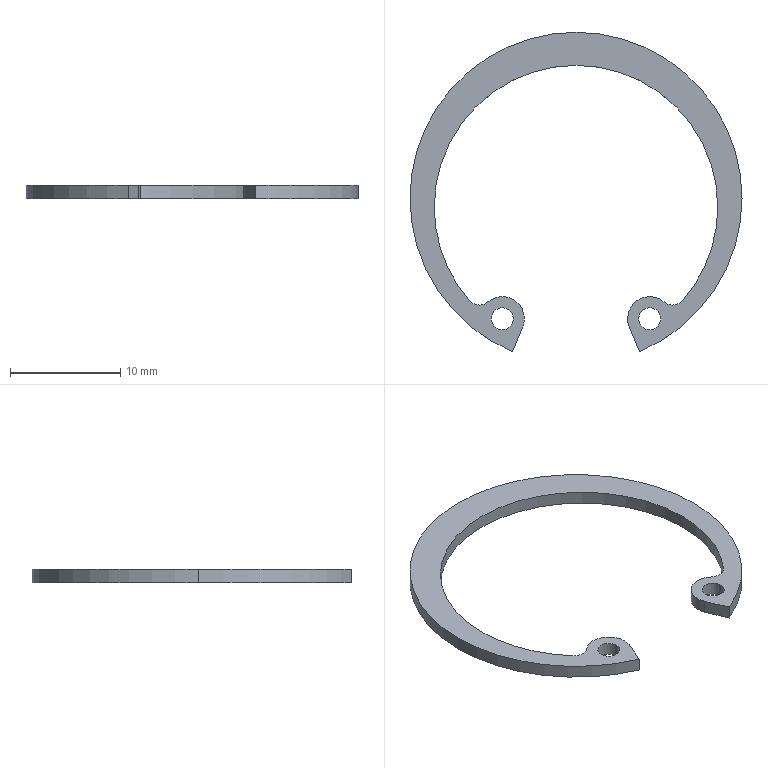Part | SolidWorks | features BaseBody 1 | 1 solid | 19 faces | box 30.1 x 28.954 x 1.2 mm | volume 227.232 mm3 | cylinder 15 | plane 4 | commonest cylinder face diameters 2 x4 4 x3 25.7 x3 30.1 x3 2.4 x2
STEP:
#1=CARTESIAN_POINT('',(15.05,0.,-1.2));
#2=VERTEX_POINT('',#1);
#3=CARTESIAN_POINT('',(-15.05,0.,-1.2));
#4=VERTEX_POINT('',#3);
#5=CARTESIAN_POINT('',(0.,0.,-1.2));
#6=DIRECTION('',(0.,0.,1.));
#7=DIRECTION('',(1.,0.,0.));
#8=AXIS2_PLACEMENT_3D('',#5,#6,#7);
#9=CIRCLE('',#8,15.05);
#10=EDGE_CURVE('',#2,#4,#9,.T.);
#11=ORIENTED_EDGE('',*,*,#10,.T.);
#12=CARTESIAN_POINT('',(-15.05,0.,0.));
#13=VERTEX_POINT('',#12);
#14=CARTESIAN_POINT('',(-15.05,0.,-1.2));
#15=DIRECTION('',(0.,0.,1.));
#16=VECTOR('',#15,1000.);
#17=LINE('',#14,#16);
#18=EDGE_CURVE('',#4,#13,#17,.T.);
#19=ORIENTED_EDGE('',*,*,#18,.T.);
#20=CARTESIAN_POINT('',(15.05,0.,0.));
#21=VERTEX_POINT('',#20);
#22=CARTESIAN_POINT('',(0.,0.,0.));
#23=DIRECTION('',(0.,0.,-1.));
#24=DIRECTION('',(1.,0.,0.));
#25=AXIS2_PLACEMENT_3D('',#22,#23,#24);
#26=CIRCLE('',#25,15.05);
#27=EDGE_CURVE('',#13,#21,#26,.T.);
#28=ORIENTED_EDGE('',*,*,#27,.T.);
#29=CARTESIAN_POINT('',(15.05,0.,-1.2));
#30=DIRECTION('',(0.,0.,1.));
#31=VECTOR('',#30,1000.);
#32=LINE('',#29,#31);
#33=EDGE_CURVE('',#2,#21,#32,.T.);
#34=ORIENTED_EDGE('',*,*,#33,.F.);
#35=EDGE_LOOP('',(#11,#19,#28,#34));
#36=FACE_OUTER_BOUND('',#35,.T.);
#37=CARTESIAN_POINT('',(0.,0.,-1.2));
#38=DIRECTION('',(0.,0.,1.));
#39=DIRECTION('',(1.,0.,0.));
#40=AXIS2_PLACEMENT_3D('',#37,#38,#39);
#41=CYLINDRICAL_SURFACE('',#40,15.05);
#42=ADVANCED_FACE('',(#36),#41,.T.);
#43=CARTESIAN_POINT('',(5.759,-13.904,-1.2));
#44=VERTEX_POINT('',#43);
#45=CARTESIAN_POINT('',(0.,0.,-1.2));
#46=DIRECTION('',(0.,0.,1.));
#47=DIRECTION('',(1.,0.,0.));
#48=AXIS2_PLACEMENT_3D('',#45,#46,#47);
#49=CIRCLE('',#48,15.05);
#50=EDGE_CURVE('',#44,#2,#49,.T.);
#51=ORIENTED_EDGE('',*,*,#50,.T.);
#52=ORIENTED_EDGE('',*,*,#33,.T.);
#53=CARTESIAN_POINT('',(5.759,-13.904,0.));
#54=VERTEX_POINT('',#53);
#55=CARTESIAN_POINT('',(0.,0.,0.));
#56=DIRECTION('',(0.,0.,-1.));
#57=DIRECTION('',(1.,0.,0.));
#58=AXIS2_PLACEMENT_3D('',#55,#56,#57);
#59=CIRCLE('',#58,15.05);
#60=EDGE_CURVE('',#21,#54,#59,.T.);
#61=ORIENTED_EDGE('',*,*,#60,.T.);
#62=CARTESIAN_POINT('',(5.759,-13.904,-1.2));
#63=DIRECTION('',(0.,0.,-1.));
#64=VECTOR('',#63,1000.);
#65=LINE('',#62,#64);
#66=EDGE_CURVE('',#54,#44,#65,.T.);
#67=ORIENTED_EDGE('',*,*,#66,.T.);
#68=EDGE_LOOP('',(#51,#52,#61,#67));
#69=FACE_OUTER_BOUND('',#68,.T.);
#70=CARTESIAN_POINT('',(0.,0.,-1.2));
#71=DIRECTION('',(0.,0.,1.));
#72=DIRECTION('',(1.,0.,0.));
#73=AXIS2_PLACEMENT_3D('',#70,#71,#72);
#74=CYLINDRICAL_SURFACE('',#73,15.05);
#75=ADVANCED_FACE('',(#69),#74,.T.);
#76=CARTESIAN_POINT('',(-9.663,-9.27,-1.2));
#77=VERTEX_POINT('',#76);
#78=CARTESIAN_POINT('',(-12.85,-0.8,-1.2));
#79=VERTEX_POINT('',#78);
#80=CARTESIAN_POINT('',(0.,-0.8,-1.2));
#81=DIRECTION('',(0.,0.,-1.));
#82=DIRECTION('',(1.,0.,0.));
#83=AXIS2_PLACEMENT_3D('',#80,#81,#82);
#84=CIRCLE('',#83,12.85);
#85=EDGE_CURVE('',#77,#79,#84,.T.);
#86=ORIENTED_EDGE('',*,*,#85,.T.);
#87=CARTESIAN_POINT('',(-12.85,-0.8,0.));
#88=VERTEX_POINT('',#87);
#89=CARTESIAN_POINT('',(-12.85,-0.8,-1.2));
#90=DIRECTION('',(0.,0.,1.));
#91=VECTOR('',#90,1000.);
#92=LINE('',#89,#91);
#93=EDGE_CURVE('',#79,#88,#92,.T.);
#94=ORIENTED_EDGE('',*,*,#93,.T.);
#95=CARTESIAN_POINT('',(-9.663,-9.27,0.));
#96=VERTEX_POINT('',#95);
#97=CARTESIAN_POINT('',(0.,-0.8,0.));
#98=DIRECTION('',(0.,0.,-1.));
#99=DIRECTION('',(1.,0.,0.));
#100=AXIS2_PLACEMENT_3D('',#97,#98,#99);
#101=CIRCLE('',#100,12.85);
#102=EDGE_CURVE('',#96,#88,#101,.T.);
#103=ORIENTED_EDGE('',*,*,#102,.F.);
#104=CARTESIAN_POINT('',(-9.663,-9.27,-1.2));
#105=DIRECTION('',(0.,0.,1.));
#106=VECTOR('',#105,1000.);
#107=LINE('',#104,#106);
#108=EDGE_CURVE('',#77,#96,#107,.T.);
#109=ORIENTED_EDGE('',*,*,#108,.F.);
#110=EDGE_LOOP('',(#86,#94,#103,#109));
#111=FACE_OUTER_BOUND('',#110,.T.);
#112=CARTESIAN_POINT('',(0.,-0.8,-1.2));
#113=DIRECTION('',(0.,0.,1.));
#114=DIRECTION('',(1.,0.,0.));
#115=AXIS2_PLACEMENT_3D('',#112,#113,#114);
#116=CYLINDRICAL_SURFACE('',#115,12.85);
#117=ADVANCED_FACE('',(#111),#116,.F.);
#118=ORIENTED_EDGE('',*,*,#93,.F.);
#119=CARTESIAN_POINT('',(12.85,-0.8,-1.2));
#120=VERTEX_POINT('',#119);
#121=CARTESIAN_POINT('',(0.,-0.8,-1.2));
#122=DIRECTION('',(0.,0.,-1.));
#123=DIRECTION('',(1.,0.,0.));
#124=AXIS2_PLACEMENT_3D('',#121,#122,#123);
#125=CIRCLE('',#124,12.85);
#126=EDGE_CURVE('',#79,#120,#125,.T.);
#127=ORIENTED_EDGE('',*,*,#126,.T.);
#128=CARTESIAN_POINT('',(12.85,-0.8,0.));
#129=VERTEX_POINT('',#128);
#130=CARTESIAN_POINT('',(12.85,-0.8,-1.2));
#131=DIRECTION('',(0.,0.,1.));
#132=VECTOR('',#131,1000.);
#133=LINE('',#130,#132);
#134=EDGE_CURVE('',#120,#129,#133,.T.);
#135=ORIENTED_EDGE('',*,*,#134,.T.);
#136=CARTESIAN_POINT('',(0.,-0.8,0.));
#137=DIRECTION('',(0.,0.,-1.));
#138=DIRECTION('',(1.,0.,0.));
#139=AXIS2_PLACEMENT_3D('',#136,#137,#138);
#140=CIRCLE('',#139,12.85);
#141=EDGE_CURVE('',#88,#129,#140,.T.);
#142=ORIENTED_EDGE('',*,*,#141,.F.);
#143=EDGE_LOOP('',(#118,#127,#135,#142));
#144=FACE_OUTER_BOUND('',#143,.T.);
#145=CARTESIAN_POINT('',(0.,-0.8,-1.2));
#146=DIRECTION('',(0.,0.,1.));
#147=DIRECTION('',(1.,0.,0.));
#148=AXIS2_PLACEMENT_3D('',#145,#146,#147);
#149=CYLINDRICAL_SURFACE('',#148,12.85);
#150=ADVANCED_FACE('',(#144),#149,.F.);
#151=CARTESIAN_POINT('',(-4.838,-11.68,-1.2));
#152=VERTEX_POINT('',#151);
#153=CARTESIAN_POINT('',(-4.686,-10.915,-1.2));
#154=VERTEX_POINT('',#153);
#155=CARTESIAN_POINT('',(-6.686,-10.915,-1.2));
#156=DIRECTION('',(0.,0.,1.));
#157=DIRECTION('',(1.,0.,0.));
#158=AXIS2_PLACEMENT_3D('',#155,#156,#157);
#159=CIRCLE('',#158,2.);
#160=EDGE_CURVE('',#152,#154,#159,.T.);
#161=ORIENTED_EDGE('',*,*,#160,.T.);
#162=CARTESIAN_POINT('',(-4.686,-10.915,0.));
#163=VERTEX_POINT('',#162);
#164=CARTESIAN_POINT('',(-4.686,-10.915,-1.2));
#165=DIRECTION('',(0.,0.,1.));
#166=VECTOR('',#165,1000.);
#167=LINE('',#164,#166);
#168=EDGE_CURVE('',#154,#163,#167,.T.);
#169=ORIENTED_EDGE('',*,*,#168,.T.);
#170=CARTESIAN_POINT('',(-4.838,-11.68,0.));
#171=VERTEX_POINT('',#170);
#172=CARTESIAN_POINT('',(-6.686,-10.915,0.));
#173=DIRECTION('',(0.,0.,-1.));
#174=DIRECTION('',(1.,0.,0.));
#175=AXIS2_PLACEMENT_3D('',#172,#173,#174);
#176=CIRCLE('',#175,2.);
#177=EDGE_CURVE('',#163,#171,#176,.T.);
#178=ORIENTED_EDGE('',*,*,#177,.T.);
#179=CARTESIAN_POINT('',(-4.838,-11.68,-1.2));
#180=DIRECTION('',(0.,0.,-1.));
#181=VECTOR('',#180,1000.);
#182=LINE('',#179,#181);
#183=EDGE_CURVE('',#171,#152,#182,.T.);
#184=ORIENTED_EDGE('',*,*,#183,.T.);
#185=EDGE_LOOP('',(#161,#169,#178,#184));
#186=FACE_OUTER_BOUND('',#185,.T.);
#187=CARTESIAN_POINT('',(-6.686,-10.915,-1.2));
#188=DIRECTION('',(0.,0.,1.));
#189=DIRECTION('',(1.,0.,0.));
#190=AXIS2_PLACEMENT_3D('',#187,#188,#189);
#191=CYLINDRICAL_SURFACE('',#190,2.);
#192=ADVANCED_FACE('',(#186),#191,.T.);
#193=CARTESIAN_POINT('',(7.686,-10.915,-1.2));
#194=VERTEX_POINT('',#193);
#195=CARTESIAN_POINT('',(5.686,-10.915,-1.2));
#196=VERTEX_POINT('',#195);
#197=CARTESIAN_POINT('',(6.686,-10.915,-1.2));
#198=DIRECTION('',(0.,0.,-1.));
#199=DIRECTION('',(1.,0.,0.));
#200=AXIS2_PLACEMENT_3D('',#197,#198,#199);
#201=CIRCLE('',#200,1.);
#202=EDGE_CURVE('',#194,#196,#201,.T.);
#203=ORIENTED_EDGE('',*,*,#202,.T.);
#204=CARTESIAN_POINT('',(5.686,-10.915,0.));
#205=VERTEX_POINT('',#204);
#206=CARTESIAN_POINT('',(5.686,-10.915,-1.2));
#207=DIRECTION('',(0.,0.,1.));
#208=VECTOR('',#207,1000.);
#209=LINE('',#206,#208);
#210=EDGE_CURVE('',#196,#205,#209,.T.);
#211=ORIENTED_EDGE('',*,*,#210,.T.);
#212=CARTESIAN_POINT('',(7.686,-10.915,0.));
#213=VERTEX_POINT('',#212);
#214=CARTESIAN_POINT('',(6.686,-10.915,0.));
#215=DIRECTION('',(0.,0.,-1.));
#216=DIRECTION('',(1.,0.,0.));
#217=AXIS2_PLACEMENT_3D('',#214,#215,#216);
#218=CIRCLE('',#217,1.);
#219=EDGE_CURVE('',#213,#205,#218,.T.);
#220=ORIENTED_EDGE('',*,*,#219,.F.);
#221=CARTESIAN_POINT('',(7.686,-10.915,-1.2));
#222=DIRECTION('',(0.,0.,1.));
#223=VECTOR('',#222,1000.);
#224=LINE('',#221,#223);
#225=EDGE_CURVE('',#194,#213,#224,.T.);
#226=ORIENTED_EDGE('',*,*,#225,.F.);
#227=EDGE_LOOP('',(#203,#211,#220,#226));
#228=FACE_OUTER_BOUND('',#227,.T.);
#229=CARTESIAN_POINT('',(6.686,-10.915,-1.2));
#230=DIRECTION('',(0.,0.,1.));
#231=DIRECTION('',(1.,0.,0.));
#232=AXIS2_PLACEMENT_3D('',#229,#230,#231);
#233=CYLINDRICAL_SURFACE('',#232,1.);
#234=ADVANCED_FACE('',(#228),#233,.F.);
#235=CARTESIAN_POINT('',(-5.686,-10.915,-1.2));
#236=VERTEX_POINT('',#235);
#237=CARTESIAN_POINT('',(-7.686,-10.915,-1.2));
#238=VERTEX_POINT('',#237);
#239=CARTESIAN_POINT('',(-6.686,-10.915,-1.2));
#240=DIRECTION('',(0.,0.,-1.));
#241=DIRECTION('',(1.,0.,0.));
#242=AXIS2_PLACEMENT_3D('',#239,#240,#241);
#243=CIRCLE('',#242,1.);
#244=EDGE_CURVE('',#236,#238,#243,.T.);
#245=ORIENTED_EDGE('',*,*,#244,.T.);
#246=CARTESIAN_POINT('',(-7.686,-10.915,0.));
#247=VERTEX_POINT('',#246);
#248=CARTESIAN_POINT('',(-7.686,-10.915,-1.2));
#249=DIRECTION('',(0.,0.,1.));
#250=VECTOR('',#249,1000.);
#251=LINE('',#248,#250);
#252=EDGE_CURVE('',#238,#247,#251,.T.);
#253=ORIENTED_EDGE('',*,*,#252,.T.);
#254=CARTESIAN_POINT('',(-5.686,-10.915,0.));
#255=VERTEX_POINT('',#254);
#256=CARTESIAN_POINT('',(-6.686,-10.915,0.));
#257=DIRECTION('',(0.,0.,-1.));
#258=DIRECTION('',(1.,0.,0.));
#259=AXIS2_PLACEMENT_3D('',#256,#257,#258);
#260=CIRCLE('',#259,1.);
#261=EDGE_CURVE('',#255,#247,#260,.T.);
#262=ORIENTED_EDGE('',*,*,#261,.F.);
#263=CARTESIAN_POINT('',(-5.686,-10.915,-1.2));
#264=DIRECTION('',(0.,0.,1.));
#265=VECTOR('',#264,1000.);
#266=LINE('',#263,#265);
#267=EDGE_CURVE('',#236,#255,#266,.T.);
#268=ORIENTED_EDGE('',*,*,#267,.F.);
#269=EDGE_LOOP('',(#245,#253,#262,#268));
#270=FACE_OUTER_BOUND('',#269,.T.);
#271=CARTESIAN_POINT('',(-6.686,-10.915,-1.2));
#272=DIRECTION('',(0.,0.,1.));
#273=DIRECTION('',(1.,0.,0.));
#274=AXIS2_PLACEMENT_3D('',#271,#272,#273);
#275=CYLINDRICAL_SURFACE('',#274,1.);
#276=ADVANCED_FACE('',(#270),#275,.F.);
#277=CARTESIAN_POINT('',(4.838,-11.68,-1.2));
#278=VERTEX_POINT('',#277);
#279=CARTESIAN_POINT('',(4.838,-11.68,-1.2));
#280=DIRECTION('',(0.3827,-0.9239,0.));
#281=VECTOR('',#280,1000.);
#282=LINE('',#279,#281);
#283=EDGE_CURVE('',#278,#44,#282,.T.);
#284=ORIENTED_EDGE('',*,*,#283,.F.);
#285=CARTESIAN_POINT('',(7.983,-9.393,-1.2));
#286=VERTEX_POINT('',#285);
#287=CARTESIAN_POINT('',(6.686,-10.915,-1.2));
#288=DIRECTION('',(0.,0.,1.));
#289=DIRECTION('',(1.,0.,0.));
#290=AXIS2_PLACEMENT_3D('',#287,#288,#289);
#291=CIRCLE('',#290,2.);
#292=EDGE_CURVE('',#286,#278,#291,.T.);
#293=ORIENTED_EDGE('',*,*,#292,.F.);
#294=CARTESIAN_POINT('',(9.663,-9.27,-1.2));
#295=VERTEX_POINT('',#294);
#296=CARTESIAN_POINT('',(8.761,-8.479,-1.2));
#297=DIRECTION('',(0.,0.,-1.));
#298=DIRECTION('',(1.,0.,0.));
#299=AXIS2_PLACEMENT_3D('',#296,#297,#298);
#300=CIRCLE('',#299,1.2);
#301=EDGE_CURVE('',#295,#286,#300,.T.);
#302=ORIENTED_EDGE('',*,*,#301,.F.);
#303=CARTESIAN_POINT('',(0.,-0.8,-1.2));
#304=DIRECTION('',(0.,0.,-1.));
#305=DIRECTION('',(1.,0.,0.));
#306=AXIS2_PLACEMENT_3D('',#303,#304,#305);
#307=CIRCLE('',#306,12.85);
#308=EDGE_CURVE('',#120,#295,#307,.T.);
#309=ORIENTED_EDGE('',*,*,#308,.F.);
#310=ORIENTED_EDGE('',*,*,#126,.F.);
#311=ORIENTED_EDGE('',*,*,#85,.F.);
#312=CARTESIAN_POINT('',(-7.983,-9.393,-1.2));
#313=VERTEX_POINT('',#312);
#314=CARTESIAN_POINT('',(-8.761,-8.479,-1.2));
#315=DIRECTION('',(0.,0.,-1.));
#316=DIRECTION('',(1.,0.,0.));
#317=AXIS2_PLACEMENT_3D('',#314,#315,#316);
#318=CIRCLE('',#317,1.2);
#319=EDGE_CURVE('',#313,#77,#318,.T.);
#320=ORIENTED_EDGE('',*,*,#319,.F.);
#321=CARTESIAN_POINT('',(-6.686,-10.915,-1.2));
#322=DIRECTION('',(0.,0.,1.));
#323=DIRECTION('',(1.,0.,0.));
#324=AXIS2_PLACEMENT_3D('',#321,#322,#323);
#325=CIRCLE('',#324,2.);
#326=EDGE_CURVE('',#154,#313,#325,.T.);
#327=ORIENTED_EDGE('',*,*,#326,.F.);
#328=ORIENTED_EDGE('',*,*,#160,.F.);
#329=CARTESIAN_POINT('',(-5.759,-13.904,-1.2));
#330=VERTEX_POINT('',#329);
#331=CARTESIAN_POINT('',(-5.759,-13.904,-1.2));
#332=DIRECTION('',(0.3827,0.9239,0.));
#333=VECTOR('',#332,1000.);
#334=LINE('',#331,#333);
#335=EDGE_CURVE('',#330,#152,#334,.T.);
#336=ORIENTED_EDGE('',*,*,#335,.F.);
#337=CARTESIAN_POINT('',(0.,0.,-1.2));
#338=DIRECTION('',(0.,0.,1.));
#339=DIRECTION('',(1.,0.,0.));
#340=AXIS2_PLACEMENT_3D('',#337,#338,#339);
#341=CIRCLE('',#340,15.05);
#342=EDGE_CURVE('',#4,#330,#341,.T.);
#343=ORIENTED_EDGE('',*,*,#342,.F.);
#344=ORIENTED_EDGE('',*,*,#10,.F.);
#345=ORIENTED_EDGE('',*,*,#50,.F.);
#346=EDGE_LOOP('',(#284,#293,#302,#309,#310,#311,#320,#327,#328,#336,#343,#344,#345));
#347=FACE_OUTER_BOUND('',#346,.T.);
#348=ORIENTED_EDGE('',*,*,#202,.F.);
#349=CARTESIAN_POINT('',(6.686,-10.915,-1.2));
#350=DIRECTION('',(0.,0.,-1.));
#351=DIRECTION('',(1.,0.,0.));
#352=AXIS2_PLACEMENT_3D('',#349,#350,#351);
#353=CIRCLE('',#352,1.);
#354=EDGE_CURVE('',#196,#194,#353,.T.);
#355=ORIENTED_EDGE('',*,*,#354,.F.);
#356=EDGE_LOOP('',(#348,#355));
#357=FACE_BOUND('',#356,.T.);
#358=ORIENTED_EDGE('',*,*,#244,.F.);
#359=CARTESIAN_POINT('',(-6.686,-10.915,-1.2));
#360=DIRECTION('',(0.,0.,-1.));
#361=DIRECTION('',(1.,0.,0.));
#362=AXIS2_PLACEMENT_3D('',#359,#360,#361);
#363=CIRCLE('',#362,1.);
#364=EDGE_CURVE('',#238,#236,#363,.T.);
#365=ORIENTED_EDGE('',*,*,#364,.F.);
#366=EDGE_LOOP('',(#358,#365));
#367=FACE_BOUND('',#366,.T.);
#368=CARTESIAN_POINT('',(0.,0.,-1.2));
#369=DIRECTION('',(0.,0.,1.));
#370=DIRECTION('',(1.,0.,0.));
#371=AXIS2_PLACEMENT_3D('',#368,#369,#370);
#372=PLANE('',#371);
#373=ADVANCED_FACE('',(#347,#357,#367),#372,.F.);
#374=ORIENTED_EDGE('',*,*,#18,.F.);
#375=ORIENTED_EDGE('',*,*,#342,.T.);
#376=CARTESIAN_POINT('',(-5.759,-13.904,0.));
#377=VERTEX_POINT('',#376);
#378=CARTESIAN_POINT('',(-5.759,-13.904,-1.2));
#379=DIRECTION('',(0.,0.,-1.));
#380=VECTOR('',#379,1000.);
#381=LINE('',#378,#380);
#382=EDGE_CURVE('',#377,#330,#381,.T.);
#383=ORIENTED_EDGE('',*,*,#382,.F.);
#384=CARTESIAN_POINT('',(0.,0.,0.));
#385=DIRECTION('',(0.,0.,-1.));
#386=DIRECTION('',(1.,0.,0.));
#387=AXIS2_PLACEMENT_3D('',#384,#385,#386);
#388=CIRCLE('',#387,15.05);
#389=EDGE_CURVE('',#377,#13,#388,.T.);
#390=ORIENTED_EDGE('',*,*,#389,.T.);
#391=EDGE_LOOP('',(#374,#375,#383,#390));
#392=FACE_OUTER_BOUND('',#391,.T.);
#393=CARTESIAN_POINT('',(0.,0.,-1.2));
#394=DIRECTION('',(0.,0.,1.));
#395=DIRECTION('',(1.,0.,0.));
#396=AXIS2_PLACEMENT_3D('',#393,#394,#395);
#397=CYLINDRICAL_SURFACE('',#396,15.05);
#398=ADVANCED_FACE('',(#392),#397,.T.);
#399=ORIENTED_EDGE('',*,*,#283,.T.);
#400=ORIENTED_EDGE('',*,*,#66,.F.);
#401=CARTESIAN_POINT('',(4.838,-11.68,0.));
#402=VERTEX_POINT('',#401);
#403=CARTESIAN_POINT('',(4.838,-11.68,0.));
#404=DIRECTION('',(-0.3827,0.9239,0.));
#405=VECTOR('',#404,1000.);
#406=LINE('',#403,#405);
#407=EDGE_CURVE('',#54,#402,#406,.T.);
#408=ORIENTED_EDGE('',*,*,#407,.T.);
#409=CARTESIAN_POINT('',(4.838,-11.68,-1.2));
#410=DIRECTION('',(0.,0.,-1.));
#411=VECTOR('',#410,1000.);
#412=LINE('',#409,#411);
#413=EDGE_CURVE('',#402,#278,#412,.T.);
#414=ORIENTED_EDGE('',*,*,#413,.T.);
#415=EDGE_LOOP('',(#399,#400,#408,#414));
#416=FACE_OUTER_BOUND('',#415,.T.);
#417=CARTESIAN_POINT('',(4.838,-11.68,-1.2));
#418=DIRECTION('',(-0.9239,-0.3827,0.));
#419=DIRECTION('',(0.3827,-0.9239,0.));
#420=AXIS2_PLACEMENT_3D('',#417,#418,#419);
#421=PLANE('',#420);
#422=ADVANCED_FACE('',(#416),#421,.T.);
#423=ORIENTED_EDGE('',*,*,#292,.T.);
#424=ORIENTED_EDGE('',*,*,#413,.F.);
#425=CARTESIAN_POINT('',(7.983,-9.393,0.));
#426=VERTEX_POINT('',#425);
#427=CARTESIAN_POINT('',(6.686,-10.915,0.));
#428=DIRECTION('',(0.,0.,-1.));
#429=DIRECTION('',(1.,0.,0.));
#430=AXIS2_PLACEMENT_3D('',#427,#428,#429);
#431=CIRCLE('',#430,2.);
#432=EDGE_CURVE('',#402,#426,#431,.T.);
#433=ORIENTED_EDGE('',*,*,#432,.T.);
#434=CARTESIAN_POINT('',(7.983,-9.393,-1.2));
#435=DIRECTION('',(0.,0.,-1.));
#436=VECTOR('',#435,1000.);
#437=LINE('',#434,#436);
#438=EDGE_CURVE('',#426,#286,#437,.T.);
#439=ORIENTED_EDGE('',*,*,#438,.T.);
#440=EDGE_LOOP('',(#423,#424,#433,#439));
#441=FACE_OUTER_BOUND('',#440,.T.);
#442=CARTESIAN_POINT('',(6.686,-10.915,-1.2));
#443=DIRECTION('',(0.,0.,1.));
#444=DIRECTION('',(1.,0.,0.));
#445=AXIS2_PLACEMENT_3D('',#442,#443,#444);
#446=CYLINDRICAL_SURFACE('',#445,2.);
#447=ADVANCED_FACE('',(#441),#446,.T.);
#448=CARTESIAN_POINT('',(9.663,-9.27,0.));
#449=VERTEX_POINT('',#448);
#450=CARTESIAN_POINT('',(9.663,-9.27,-1.2));
#451=DIRECTION('',(0.,0.,1.));
#452=VECTOR('',#451,1000.);
#453=LINE('',#450,#452);
#454=EDGE_CURVE('',#295,#449,#453,.T.);
#455=ORIENTED_EDGE('',*,*,#454,.F.);
#456=ORIENTED_EDGE('',*,*,#301,.T.);
#457=ORIENTED_EDGE('',*,*,#438,.F.);
#458=CARTESIAN_POINT('',(8.761,-8.479,0.));
#459=DIRECTION('',(0.,0.,-1.));
#460=DIRECTION('',(1.,0.,0.));
#461=AXIS2_PLACEMENT_3D('',#458,#459,#460);
#462=CIRCLE('',#461,1.2);
#463=EDGE_CURVE('',#449,#426,#462,.T.);
#464=ORIENTED_EDGE('',*,*,#463,.F.);
#465=EDGE_LOOP('',(#455,#456,#457,#464));
#466=FACE_OUTER_BOUND('',#465,.T.);
#467=CARTESIAN_POINT('',(8.761,-8.479,-1.2));
#468=DIRECTION('',(0.,0.,1.));
#469=DIRECTION('',(1.,0.,0.));
#470=AXIS2_PLACEMENT_3D('',#467,#468,#469);
#471=CYLINDRICAL_SURFACE('',#470,1.2);
#472=ADVANCED_FACE('',(#466),#471,.F.);
#473=ORIENTED_EDGE('',*,*,#134,.F.);
#474=ORIENTED_EDGE('',*,*,#308,.T.);
#475=ORIENTED_EDGE('',*,*,#454,.T.);
#476=CARTESIAN_POINT('',(0.,-0.8,0.));
#477=DIRECTION('',(0.,0.,-1.));
#478=DIRECTION('',(1.,0.,0.));
#479=AXIS2_PLACEMENT_3D('',#476,#477,#478);
#480=CIRCLE('',#479,12.85);
#481=EDGE_CURVE('',#129,#449,#480,.T.);
#482=ORIENTED_EDGE('',*,*,#481,.F.);
#483=EDGE_LOOP('',(#473,#474,#475,#482));
#484=FACE_OUTER_BOUND('',#483,.T.);
#485=CARTESIAN_POINT('',(0.,-0.8,-1.2));
#486=DIRECTION('',(0.,0.,1.));
#487=DIRECTION('',(1.,0.,0.));
#488=AXIS2_PLACEMENT_3D('',#485,#486,#487);
#489=CYLINDRICAL_SURFACE('',#488,12.85);
#490=ADVANCED_FACE('',(#484),#489,.F.);
#491=CARTESIAN_POINT('',(-7.983,-9.393,0.));
#492=VERTEX_POINT('',#491);
#493=CARTESIAN_POINT('',(-7.983,-9.393,-1.2));
#494=DIRECTION('',(0.,0.,1.));
#495=VECTOR('',#494,1000.);
#496=LINE('',#493,#495);
#497=EDGE_CURVE('',#313,#492,#496,.T.);
#498=ORIENTED_EDGE('',*,*,#497,.F.);
#499=ORIENTED_EDGE('',*,*,#319,.T.);
#500=ORIENTED_EDGE('',*,*,#108,.T.);
#501=CARTESIAN_POINT('',(-8.761,-8.479,0.));
#502=DIRECTION('',(0.,0.,-1.));
#503=DIRECTION('',(1.,0.,0.));
#504=AXIS2_PLACEMENT_3D('',#501,#502,#503);
#505=CIRCLE('',#504,1.2);
#506=EDGE_CURVE('',#492,#96,#505,.T.);
#507=ORIENTED_EDGE('',*,*,#506,.F.);
#508=EDGE_LOOP('',(#498,#499,#500,#507));
#509=FACE_OUTER_BOUND('',#508,.T.);
#510=CARTESIAN_POINT('',(-8.761,-8.479,-1.2));
#511=DIRECTION('',(0.,0.,1.));
#512=DIRECTION('',(1.,0.,0.));
#513=AXIS2_PLACEMENT_3D('',#510,#511,#512);
#514=CYLINDRICAL_SURFACE('',#513,1.2);
#515=ADVANCED_FACE('',(#509),#514,.F.);
#516=ORIENTED_EDGE('',*,*,#168,.F.);
#517=ORIENTED_EDGE('',*,*,#326,.T.);
#518=ORIENTED_EDGE('',*,*,#497,.T.);
#519=CARTESIAN_POINT('',(-6.686,-10.915,0.));
#520=DIRECTION('',(0.,0.,-1.));
#521=DIRECTION('',(1.,0.,0.));
#522=AXIS2_PLACEMENT_3D('',#519,#520,#521);
#523=CIRCLE('',#522,2.);
#524=EDGE_CURVE('',#492,#163,#523,.T.);
#525=ORIENTED_EDGE('',*,*,#524,.T.);
#526=EDGE_LOOP('',(#516,#517,#518,#525));
#527=FACE_OUTER_BOUND('',#526,.T.);
#528=CARTESIAN_POINT('',(-6.686,-10.915,-1.2));
#529=DIRECTION('',(0.,0.,1.));
#530=DIRECTION('',(1.,0.,0.));
#531=AXIS2_PLACEMENT_3D('',#528,#529,#530);
#532=CYLINDRICAL_SURFACE('',#531,2.);
#533=ADVANCED_FACE('',(#527),#532,.T.);
#534=ORIENTED_EDGE('',*,*,#335,.T.);
#535=ORIENTED_EDGE('',*,*,#183,.F.);
#536=CARTESIAN_POINT('',(-4.838,-11.68,0.));
#537=DIRECTION('',(-0.3827,-0.9239,0.));
#538=VECTOR('',#537,1000.);
#539=LINE('',#536,#538);
#540=EDGE_CURVE('',#171,#377,#539,.T.);
#541=ORIENTED_EDGE('',*,*,#540,.T.);
#542=ORIENTED_EDGE('',*,*,#382,.T.);
#543=EDGE_LOOP('',(#534,#535,#541,#542));
#544=FACE_OUTER_BOUND('',#543,.T.);
#545=CARTESIAN_POINT('',(-4.838,-11.68,-1.2));
#546=DIRECTION('',(0.9239,-0.3827,0.));
#547=DIRECTION('',(0.3827,0.9239,0.));
#548=AXIS2_PLACEMENT_3D('',#545,#546,#547);
#549=PLANE('',#548);
#550=ADVANCED_FACE('',(#544),#549,.T.);
#551=ORIENTED_EDGE('',*,*,#210,.F.);
#552=ORIENTED_EDGE('',*,*,#354,.T.);
#553=ORIENTED_EDGE('',*,*,#225,.T.);
#554=CARTESIAN_POINT('',(6.686,-10.915,0.));
#555=DIRECTION('',(0.,0.,-1.));
#556=DIRECTION('',(1.,0.,0.));
#557=AXIS2_PLACEMENT_3D('',#554,#555,#556);
#558=CIRCLE('',#557,1.);
#559=EDGE_CURVE('',#205,#213,#558,.T.);
#560=ORIENTED_EDGE('',*,*,#559,.F.);
#561=EDGE_LOOP('',(#551,#552,#553,#560));
#562=FACE_OUTER_BOUND('',#561,.T.);
#563=CARTESIAN_POINT('',(6.686,-10.915,-1.2));
#564=DIRECTION('',(0.,0.,1.));
#565=DIRECTION('',(1.,0.,0.));
#566=AXIS2_PLACEMENT_3D('',#563,#564,#565);
#567=CYLINDRICAL_SURFACE('',#566,1.);
#568=ADVANCED_FACE('',(#562),#567,.F.);
#569=ORIENTED_EDGE('',*,*,#252,.F.);
#570=ORIENTED_EDGE('',*,*,#364,.T.);
#571=ORIENTED_EDGE('',*,*,#267,.T.);
#572=CARTESIAN_POINT('',(-6.686,-10.915,0.));
#573=DIRECTION('',(0.,0.,-1.));
#574=DIRECTION('',(1.,0.,0.));
#575=AXIS2_PLACEMENT_3D('',#572,#573,#574);
#576=CIRCLE('',#575,1.);
#577=EDGE_CURVE('',#247,#255,#576,.T.);
#578=ORIENTED_EDGE('',*,*,#577,.F.);
#579=EDGE_LOOP('',(#569,#570,#571,#578));
#580=FACE_OUTER_BOUND('',#579,.T.);
#581=CARTESIAN_POINT('',(-6.686,-10.915,-1.2));
#582=DIRECTION('',(0.,0.,1.));
#583=DIRECTION('',(1.,0.,0.));
#584=AXIS2_PLACEMENT_3D('',#581,#582,#583);
#585=CYLINDRICAL_SURFACE('',#584,1.);
#586=ADVANCED_FACE('',(#580),#585,.F.);
#587=ORIENTED_EDGE('',*,*,#432,.F.);
#588=ORIENTED_EDGE('',*,*,#407,.F.);
#589=ORIENTED_EDGE('',*,*,#60,.F.);
#590=ORIENTED_EDGE('',*,*,#27,.F.);
#591=ORIENTED_EDGE('',*,*,#389,.F.);
#592=ORIENTED_EDGE('',*,*,#540,.F.);
#593=ORIENTED_EDGE('',*,*,#177,.F.);
#594=ORIENTED_EDGE('',*,*,#524,.F.);
#595=ORIENTED_EDGE('',*,*,#506,.T.);
#596=ORIENTED_EDGE('',*,*,#102,.T.);
#597=ORIENTED_EDGE('',*,*,#141,.T.);
#598=ORIENTED_EDGE('',*,*,#481,.T.);
#599=ORIENTED_EDGE('',*,*,#463,.T.);
#600=EDGE_LOOP('',(#587,#588,#589,#590,#591,#592,#593,#594,#595,#596,#597,#598,#599));
#601=FACE_OUTER_BOUND('',#600,.T.);
#602=ORIENTED_EDGE('',*,*,#219,.T.);
#603=ORIENTED_EDGE('',*,*,#559,.T.);
#604=EDGE_LOOP('',(#602,#603));
#605=FACE_BOUND('',#604,.T.);
#606=ORIENTED_EDGE('',*,*,#261,.T.);
#607=ORIENTED_EDGE('',*,*,#577,.T.);
#608=EDGE_LOOP('',(#606,#607));
#609=FACE_BOUND('',#608,.T.);
#610=CARTESIAN_POINT('',(0.,0.,0.));
#611=DIRECTION('',(0.,0.,1.));
#612=DIRECTION('',(1.,0.,0.));
#613=AXIS2_PLACEMENT_3D('',#610,#611,#612);
#614=PLANE('',#613);
#615=ADVANCED_FACE('',(#601,#605,#609),#614,.T.);
#616=CLOSED_SHELL('',(#42,#75,#117,#150,#192,#234,#276,#373,#398,#422,#447,#472,#490,#515,#533,#550,#568,#586,#615));
#617=MANIFOLD_SOLID_BREP('',#616);
#618=CARTESIAN_POINT('',(0.,0.,0.));
#619=DIRECTION('',(0.,0.,1.));
#620=DIRECTION('',(1.,0.,0.));
#621=AXIS2_PLACEMENT_3D('',#618,#619,#620);
#622=(LENGTH_UNIT()NAMED_UNIT(*)SI_UNIT(.MILLI.,.METRE.));
#623=UNCERTAINTY_MEASURE_WITH_UNIT(LENGTH_MEASURE(0.00001),#622,'','');
#624=(NAMED_UNIT(*)PLANE_ANGLE_UNIT()SI_UNIT($,.RADIAN.));
#625=(NAMED_UNIT(*)SI_UNIT($,.STERADIAN.)SOLID_ANGLE_UNIT());
#626=(GEOMETRIC_REPRESENTATION_CONTEXT(3)GLOBAL_UNCERTAINTY_ASSIGNED_CONTEXT((#623))GLOBAL_UNIT_ASSIGNED_CONTEXT((#622,#624,#625))REPRESENTATION_CONTEXT('',''));
#627=ADVANCED_BREP_SHAPE_REPRESENTATION('',(#617,#621),#626);